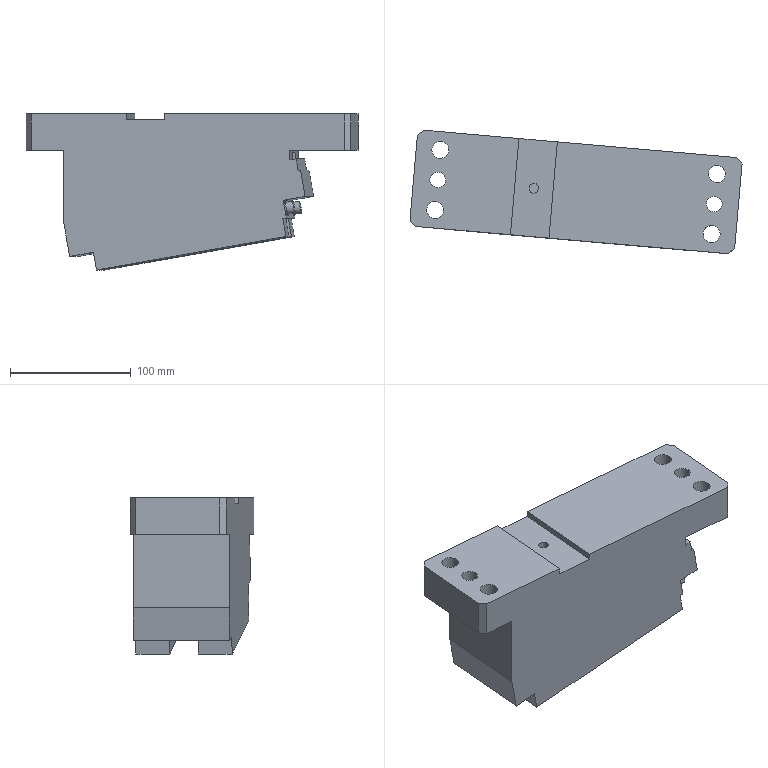Part | NX | features solid 2 | 1 solid | 114 faces | box 275.073 x 102.356 x 129.326 mm | volume 1519024 mm3 | plane 76 | cylinder 38 | commonest cylinder face diameters 10 x8 14 x8 20 x8 12.5 x4 13 x4 8 x2